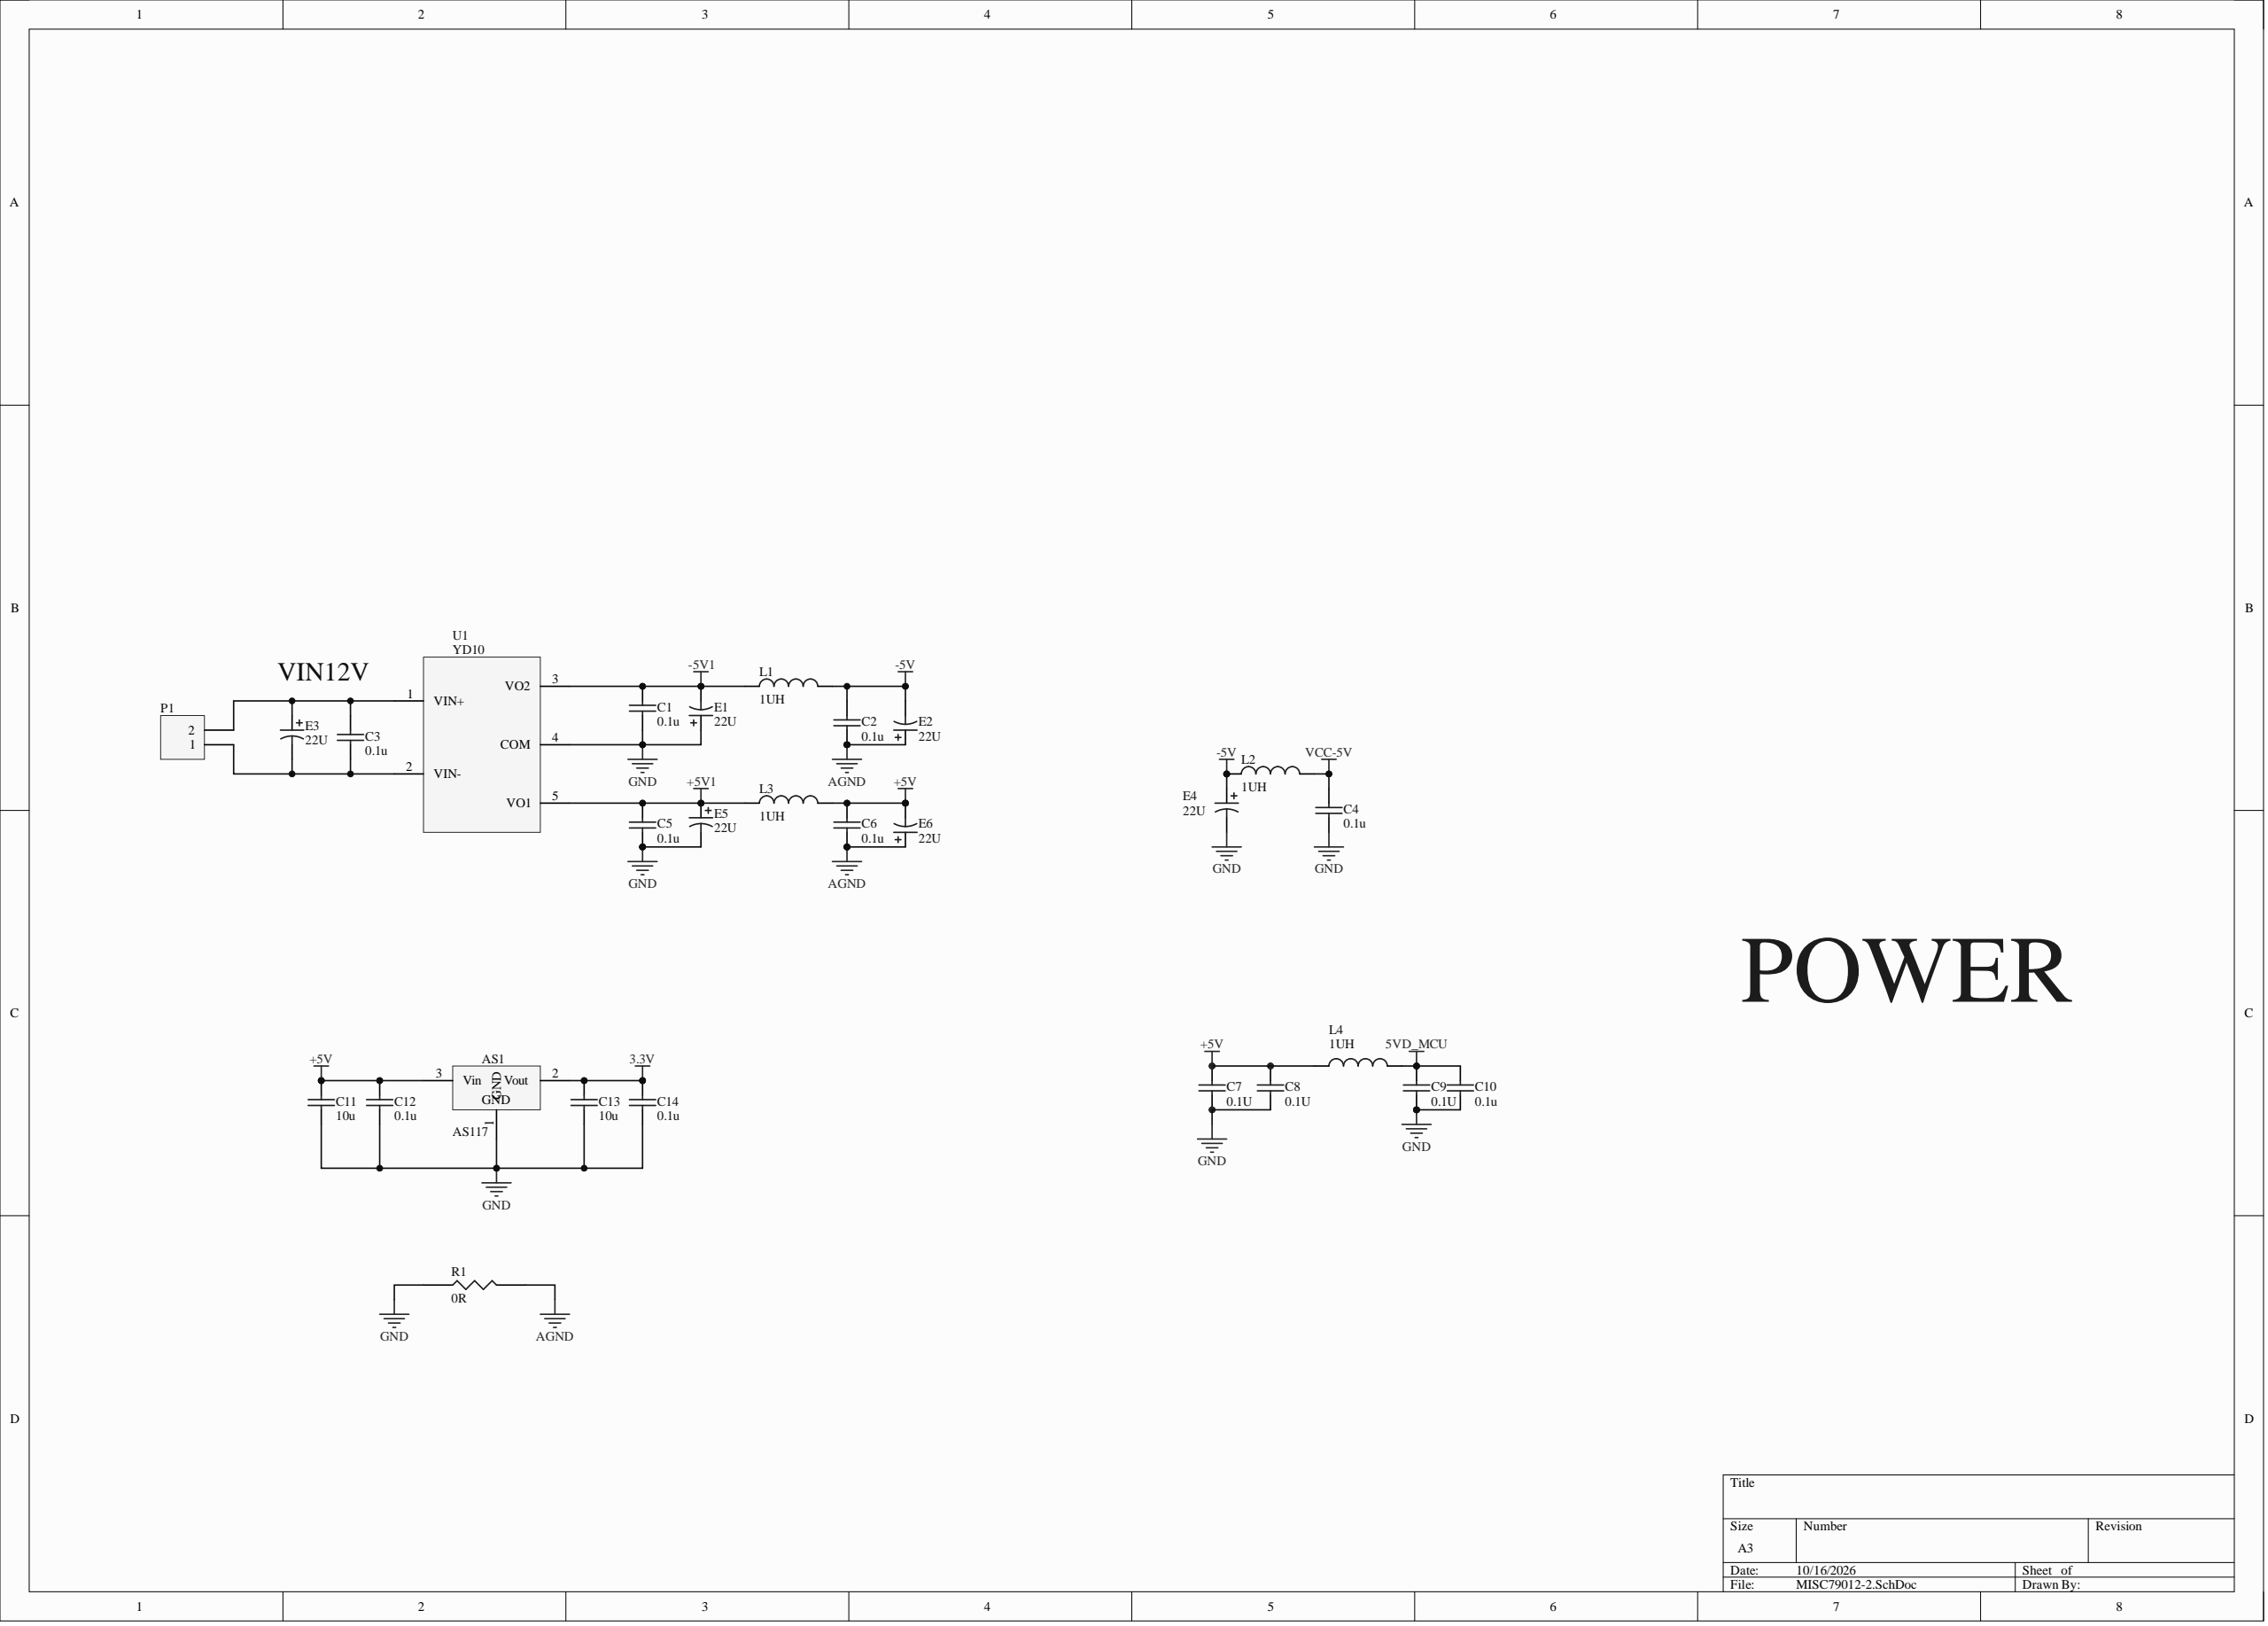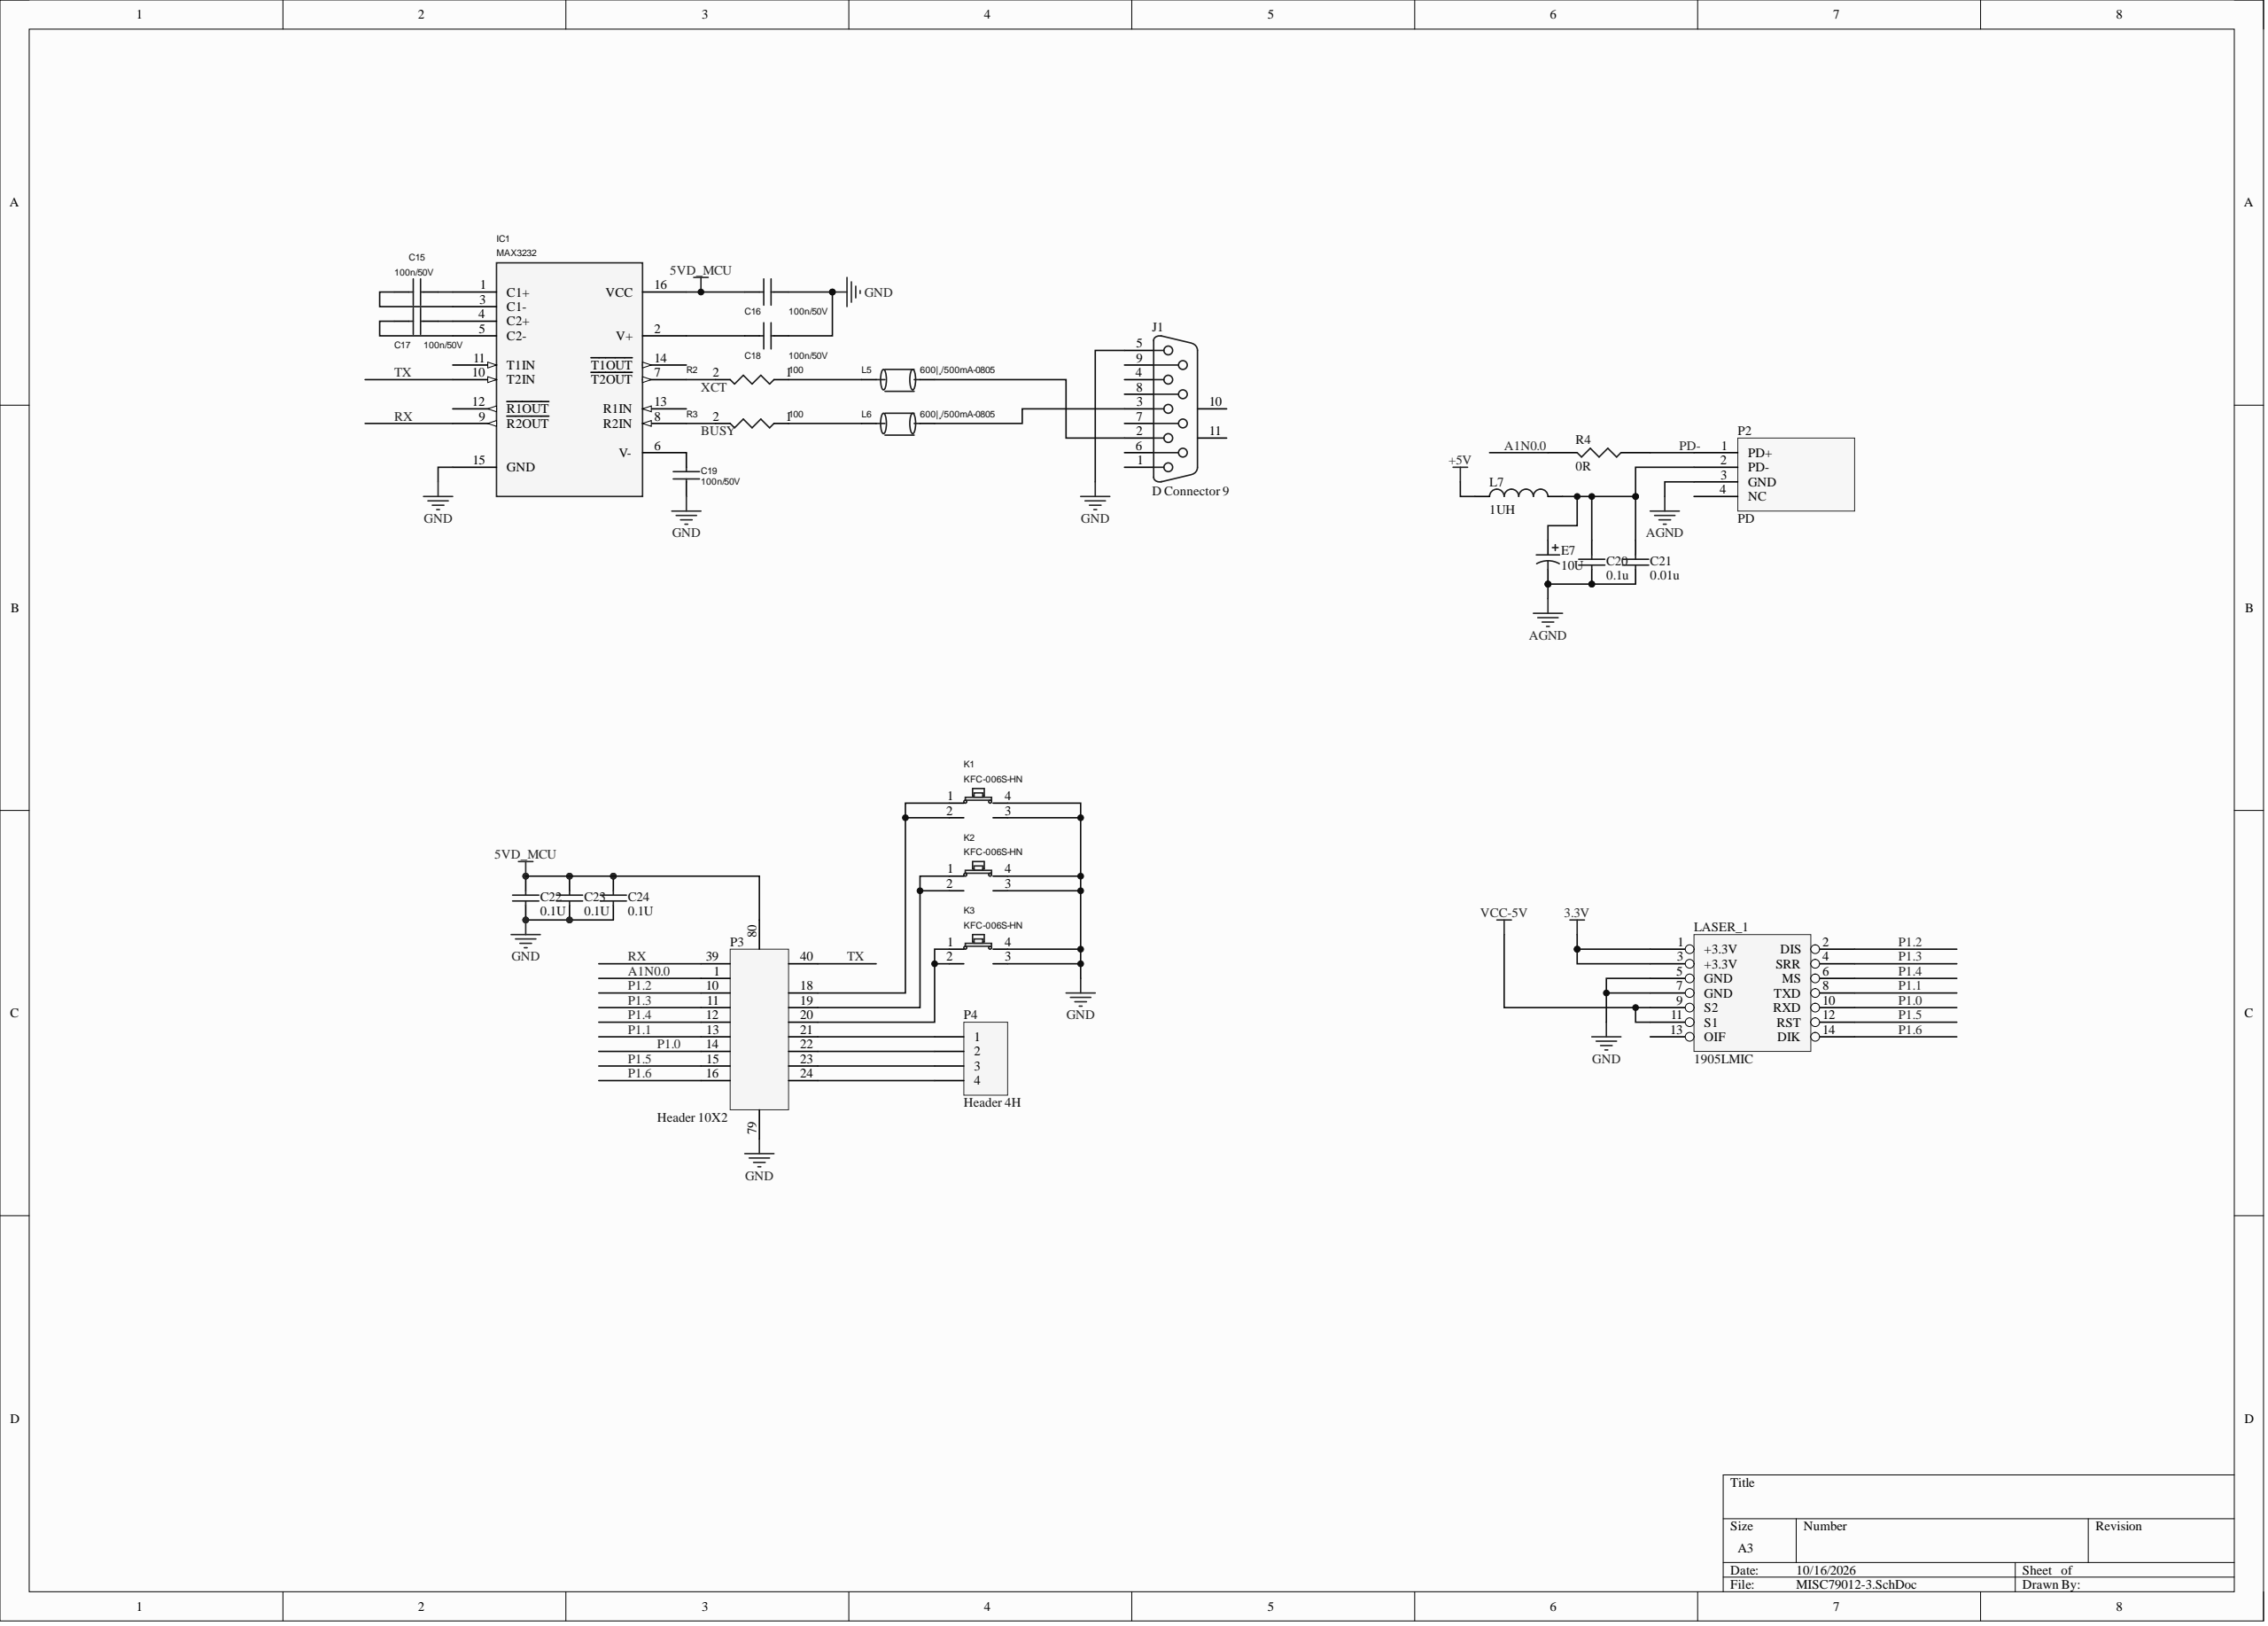Circuit board | Altium Designer | 54 parts | 42 nets
Bill of materials:
Comment,Description,Designator,Footprint,LibRef,Quantity
"AS117","Voltage Regulator","AS1","SOT223-4","Volt Reg","1"
"0.1u","Capacitor","C1, C2, C3, C4, C5, C6, C7, C8, C9, C10, C12, C14, C20, C22, C23, C24","0603","CAP","16"
"10u","Capacitor, Polarized Capacitor (Radial)","C11, C13, E7","1210","CAP, Cap Pol1","3"
"100n/50V","","C15, C16, C17, C18, C19","0603","CAPACITOR NON-POL","5"
"0.01u","Capacitor","C21","0603","CAP","1"
"22U","Polarized Capacitor (Radial)","E1, E2, E3, E4, E5, E6","1210","Cap Pol1","6"
"MAX3232","","IC1","SOIC127P600-16N","MAX3232","1"
"D Connector 9","Receptacle Assembly, 9 Position, Right Angle","J1","DSUB1.385-2H9","D Connector 9","1"
"KFC-006S-HN","","K1, K2, K3","KNOB-SMD","KNOB-SMD","3"
"1UH","","L1, L2, L3, L4, L7","0805","INDUCTOR","5"
"600|¸/500mA-0805","","L5, L6","0805","BEAD","2"
"1905LMIC","","LASER_1","CLM-107-02-H-D-K-TR","1905LMI","1"
"","Header, 2-Pin, Right Angle","P1","MKDS3_2RMI","Header 2H","1"
"PD","","P2","guang2","FDDI","1"
"Header 10X2","Header, 10-Pin, Dual row","P3","c8051","Header 10X2","1"
"Header 4H","Header, 4-Pin, Right Angle","P4","DIP-4","Header 4H","1"
"0R","","R1, R4","0603","RES1","2"
"100","","R2, R3","0603","SMDRXX_2","2"
"YD10","","U1","YD10","YD10","1"
Netlist (Protel format):
[
AS1
SOT223-4
AS117



]
[
C1
0603
0.1u



]
[
C2
0603
0.1u



]
[
C3
0603
0.1u



]
[
C4
0603
0.1u



]
[
C5
0603
0.1u



]
[
C6
0603
0.1u



]
[
C7
0603
0.1U



]
[
C8
0603
0.1U



]
[
C9
0603
0.1U



]
[
C10
0603
0.1u



]
[
C11
1210
10u



]
[
C12
0603
0.1u



]
[
C13
1210
10u



]
[
C14
0603
0.1u



]
[
C15
0603
100n/50V



]
[
C16
0603
100n/50V



]
[
C17
0603
100n/50V



]
[
C18
0603
100n/50V



]
[
C19
0603
100n/50V



]
[
C20
0603
0.1u



]
[
C21
0603
0.01u



]
[
C22
0603
0.1U



]
[
C23
0603
0.1U



]
[
C24
0603
0.1U



]
[
E1
1210
22U



]
[
E2
1210
22U



]
[
E3
1210
22U



]
[
E4
1210
22U



]
[
E5
1210
22U



]
[
E6
1210
22U



]
[
E7
1210
10U



]
[
IC1
SOIC127P600-16N
MAX3232



]
[
J1
DSUB1.385-2H9
D Connector 9



]
[
K1
KNOB-SMD
KFC-006S-HN



]
[
K2
KNOB-SMD
KFC-006S-HN



]
[
K3
KNOB-SMD
KFC-006S-HN



]
[
L1
0805
1UH



]
[
L2
0805
1UH



]
[
L3
0805
1UH



]
[
L4
0805
1UH



]
[
L5
0805
600|¸/500mA-0805



]
[
L6
0805
600|¸/500mA-0805



]
[
L7
0805
1UH



]
[
LASER_1
CLM-107-02-H-D-K-TR
1905LMIC



]
[
P1
MKDS3_2RMI




]
[
P2
guang2
PD



]
[
P3
c8051
Header 10X2



]
[
P4
DIP-4
Header 4H



]
[
R1
0603
0R



]
[
R2
0603
100



]
[
R3
0603
100



]
[
R4
0603
0R



]
[
U1
YD10
YD10



]
(
VCC-5V
C4-1
L2-2
LASER_1-9
LASER_1-11
)
(
TX
IC1-10
P3-40
)
(
RX
IC1-9
P3-39
)
(
PD-
P2-1
R4-2
)
(
P1.6
LASER_1-14
P3-16
)
(
P1.5
LASER_1-12
P3-15
)
(
P1.4
LASER_1-6
P3-12
)
(
P1.3
LASER_1-4
P3-11
)
(
P1.2
LASER_1-2
P3-10
)
(
P1.1
LASER_1-8
P3-13
)
(
P1.0
LASER_1-10
P3-14
)
(
NetP3_24
P3-24
P4-4
)
(
NetP3_23
P3-23
P4-3
)
(
NetP3_22
P3-22
P4-2
)
(
NetP3_21
P3-21
P4-1
)
(
NetL6_1
L6-1
R3-1
)
(
NetL5_1
L5-1
R2-1
)
(
NetK3_1
K3-1
K3-2
P3-20
)
(
NetK2_1
K2-1
K2-2
P3-19
)
(
NetK1_1
K1-1
K1-2
P3-18
)
(
NetJ1_3
J1-3
L6-2
)
(
NetJ1_2
J1-2
L5-2
)
(
NetIC1_8
IC1-8
R3-2
)
(
NetIC1_7
IC1-7
R2-2
)
(
NetC20_1
C20-1
C21-1
E7-1
L7-2
P2-2
)
(
NetC19_2
C19-2
IC1-6
)
(
NetC18_2
C18-2
IC1-2
)
(
NetC17_2
C17-2
IC1-5
)
(
NetC17_1
C17-1
IC1-4
)
(
NetC15_2
C15-2
IC1-3
)
(
NetC15_1
C15-1
IC1-1
)
(
NetC3_2
C3-2
E3-2
P1-1
U1-2
)
(
NetC3_1
C3-1
E3-1
P1-2
U1-1
)
(
GND
AS1-1
C1-2
C4-2
C5-2
C7-1
C8-1
C9-1
C10-2
C11-2
C12-2
C13-2
C14-2
C16-1
C18-1
C19-1
C22-1
C23-1
C24-1
E1-1
E4-2
E5-2
IC1-15
J1-5
K1-3
K1-4
K2-3
K2-4
K3-3
K3-4
LASER_1-5
LASER_1-7
P3-79
R1-2
U1-4
)
(
AGND
C2-2
C6-2
C20-2
C21-2
E2-1
E6-1
E7-2
P2-3
R1-1
)
(
A1N0.0
P3-1
R4-1
)
(
-5V1
C1-1
E1-2
L1-1
U1-3
)
(
-5V
C2-1
E2-2
E4-1
L1-2
L2-1
)
(
+5V1
C5-1
E5-1
L3-1
U1-5
)
(
+5V
AS1-3
C6-1
C7-2
C8-2
C11-1
C12-1
E6-2
L3-2
L4-2
L7-1
)
(
5VD_MCU
C9-2
C10-1
C16-2
C22-2
C23-2
C24-2
IC1-16
L4-1
P3-80
)
(
3.3V
AS1-2
C13-1
C14-1
LASER_1-1
LASER_1-3
)